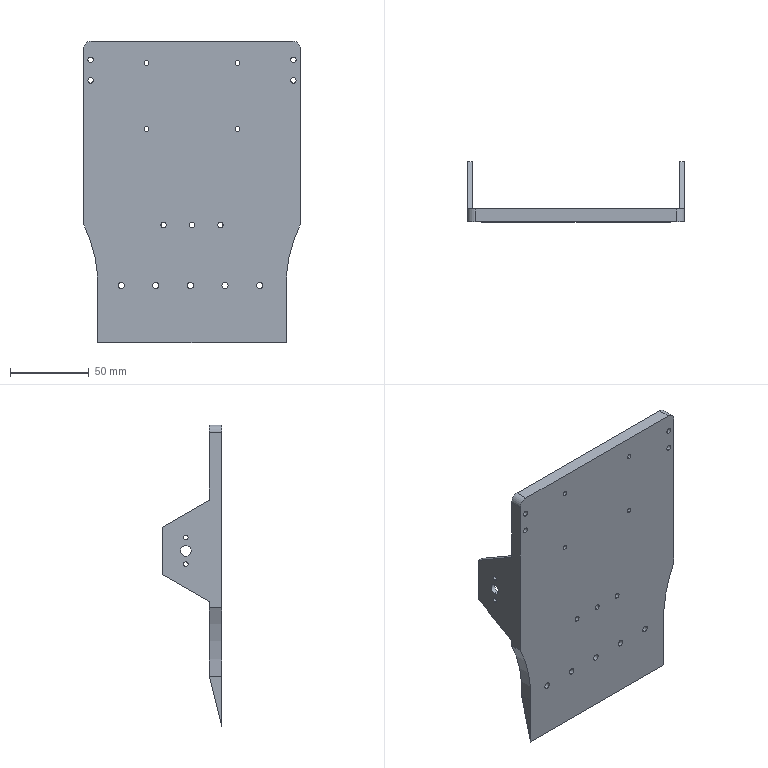Part | SolidWorks | features ICE 7, MirrorPattern 4, Extrusion 1, Fillet 1, Rib 1 | 1 solid | 64 faces | box 138 x 38 x 192 mm | volume 194346 mm3 | cylinder 48 | plane 16 | commonest cylinder face diameters 3 x16 3.5 x14 4 x10 6.8 x4 10 x2 176 x2